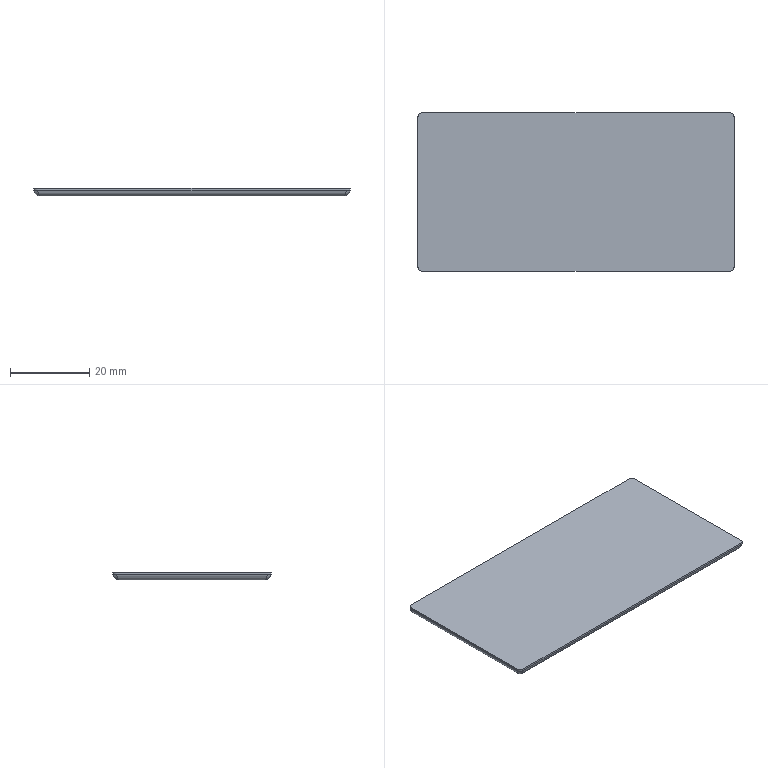Part | STEP file | Profile end cap | 1 solid | 18 faces | box 80 x 40 x 2 mm | volume 6284 mm3 | cylinder 8 | plane 6 | spline 4 | commonest cylinder face diameters 2 x4 3 x4